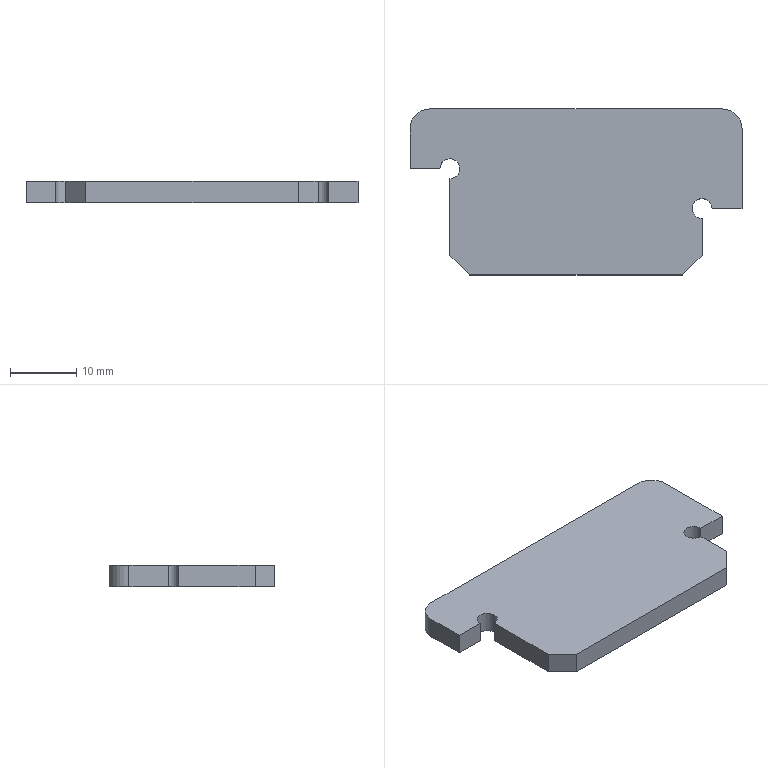Part | SolidWorks | features FlatPattern 1, SMBaseFlange 1, SheetMetal 1 | 1 solid | 17 faces | box 50 x 25 x 3.2 mm | volume 3426 mm3 | plane 12 | cylinder 5 | commonest cylinder face diameters 3 x3 6 x2
STEP:
#1=CARTESIAN_POINT('',(-86.411,-492.5,3.2));
#2=VERTEX_POINT('',#1);
#3=CARTESIAN_POINT('',(-83.411,-492.5,3.2));
#4=VERTEX_POINT('',#3);
#5=CARTESIAN_POINT('',(-84.911,-492.5,3.2));
#6=DIRECTION('',(0.,0.,-1.));
#7=DIRECTION('',(1.,0.,0.));
#8=AXIS2_PLACEMENT_3D('',#5,#6,#7);
#9=CIRCLE('',#8,1.5);
#10=EDGE_CURVE('',#2,#4,#9,.T.);
#11=ORIENTED_EDGE('',*,*,#10,.F.);
#12=CARTESIAN_POINT('',(-86.411,-492.5,0.));
#13=VERTEX_POINT('',#12);
#14=CARTESIAN_POINT('',(-86.411,-492.5,3.2));
#15=DIRECTION('',(0.,0.,-1.));
#16=VECTOR('',#15,1000.);
#17=LINE('',#14,#16);
#18=EDGE_CURVE('',#2,#13,#17,.T.);
#19=ORIENTED_EDGE('',*,*,#18,.T.);
#20=CARTESIAN_POINT('',(-83.411,-492.5,0.));
#21=VERTEX_POINT('',#20);
#22=CARTESIAN_POINT('',(-84.911,-492.5,0.));
#23=DIRECTION('',(0.,0.,-1.));
#24=DIRECTION('',(1.,0.,0.));
#25=AXIS2_PLACEMENT_3D('',#22,#23,#24);
#26=CIRCLE('',#25,1.5);
#27=EDGE_CURVE('',#13,#21,#26,.T.);
#28=ORIENTED_EDGE('',*,*,#27,.T.);
#29=CARTESIAN_POINT('',(-83.411,-492.5,3.2));
#30=DIRECTION('',(0.,0.,-1.));
#31=VECTOR('',#30,1000.);
#32=LINE('',#29,#31);
#33=EDGE_CURVE('',#4,#21,#32,.T.);
#34=ORIENTED_EDGE('',*,*,#33,.F.);
#35=EDGE_LOOP('',(#11,#19,#28,#34));
#36=FACE_OUTER_BOUND('',#35,.T.);
#37=CARTESIAN_POINT('',(-84.911,-492.5,3.2));
#38=DIRECTION('',(0.,0.,-1.));
#39=DIRECTION('',(-1.,0.,0.));
#40=AXIS2_PLACEMENT_3D('',#37,#38,#39);
#41=CYLINDRICAL_SURFACE('',#40,1.5);
#42=ADVANCED_FACE('',(#36),#41,.F.);
#43=CARTESIAN_POINT('',(-128.911,-486.5,0.));
#44=VERTEX_POINT('',#43);
#45=CARTESIAN_POINT('',(-124.411,-486.5,0.));
#46=VERTEX_POINT('',#45);
#47=CARTESIAN_POINT('',(-124.411,-486.5,0.));
#48=DIRECTION('',(1.,0.,0.));
#49=VECTOR('',#48,1000.);
#50=LINE('',#47,#49);
#51=EDGE_CURVE('',#44,#46,#50,.T.);
#52=ORIENTED_EDGE('',*,*,#51,.T.);
#53=CARTESIAN_POINT('',(-124.411,-486.5,3.2));
#54=VERTEX_POINT('',#53);
#55=CARTESIAN_POINT('',(-124.411,-486.5,3.2));
#56=DIRECTION('',(0.,0.,-1.));
#57=VECTOR('',#56,1000.);
#58=LINE('',#55,#57);
#59=EDGE_CURVE('',#54,#46,#58,.T.);
#60=ORIENTED_EDGE('',*,*,#59,.F.);
#61=CARTESIAN_POINT('',(-128.911,-486.5,3.2));
#62=VERTEX_POINT('',#61);
#63=CARTESIAN_POINT('',(-124.411,-486.5,3.2));
#64=DIRECTION('',(1.,0.,0.));
#65=VECTOR('',#64,1000.);
#66=LINE('',#63,#65);
#67=EDGE_CURVE('',#62,#54,#66,.T.);
#68=ORIENTED_EDGE('',*,*,#67,.F.);
#69=CARTESIAN_POINT('',(-128.911,-486.5,3.2));
#70=DIRECTION('',(0.,0.,-1.));
#71=VECTOR('',#70,1000.);
#72=LINE('',#69,#71);
#73=EDGE_CURVE('',#62,#44,#72,.T.);
#74=ORIENTED_EDGE('',*,*,#73,.T.);
#75=EDGE_LOOP('',(#52,#60,#68,#74));
#76=FACE_OUTER_BOUND('',#75,.T.);
#77=CARTESIAN_POINT('',(-124.411,-486.5,3.2));
#78=DIRECTION('',(0.,1.,0.));
#79=DIRECTION('',(0.,0.,1.));
#80=AXIS2_PLACEMENT_3D('',#77,#78,#79);
#81=PLANE('',#80);
#82=ADVANCED_FACE('',(#76),#81,.F.);
#83=CARTESIAN_POINT('',(-122.911,-488.,0.));
#84=VERTEX_POINT('',#83);
#85=CARTESIAN_POINT('',(-122.911,-486.5,0.));
#86=DIRECTION('',(0.,0.,-1.));
#87=DIRECTION('',(1.,0.,0.));
#88=AXIS2_PLACEMENT_3D('',#85,#86,#87);
#89=CIRCLE('',#88,1.5);
#90=EDGE_CURVE('',#46,#84,#89,.T.);
#91=ORIENTED_EDGE('',*,*,#90,.T.);
#92=CARTESIAN_POINT('',(-122.911,-488.,3.2));
#93=VERTEX_POINT('',#92);
#94=CARTESIAN_POINT('',(-122.911,-488.,3.2));
#95=DIRECTION('',(0.,0.,-1.));
#96=VECTOR('',#95,1000.);
#97=LINE('',#94,#96);
#98=EDGE_CURVE('',#93,#84,#97,.T.);
#99=ORIENTED_EDGE('',*,*,#98,.F.);
#100=CARTESIAN_POINT('',(-122.911,-486.5,3.2));
#101=DIRECTION('',(0.,0.,-1.));
#102=DIRECTION('',(1.,0.,0.));
#103=AXIS2_PLACEMENT_3D('',#100,#101,#102);
#104=CIRCLE('',#103,1.5);
#105=EDGE_CURVE('',#54,#93,#104,.T.);
#106=ORIENTED_EDGE('',*,*,#105,.F.);
#107=ORIENTED_EDGE('',*,*,#59,.T.);
#108=EDGE_LOOP('',(#91,#99,#106,#107));
#109=FACE_OUTER_BOUND('',#108,.T.);
#110=CARTESIAN_POINT('',(-122.911,-486.5,3.2));
#111=DIRECTION('',(0.,0.,-1.));
#112=DIRECTION('',(-1.,0.,0.));
#113=AXIS2_PLACEMENT_3D('',#110,#111,#112);
#114=CYLINDRICAL_SURFACE('',#113,1.5);
#115=ADVANCED_FACE('',(#109),#114,.F.);
#116=CARTESIAN_POINT('',(-122.911,-499.5,0.));
#117=VERTEX_POINT('',#116);
#118=CARTESIAN_POINT('',(-122.911,-499.5,0.));
#119=DIRECTION('',(0.,-1.,0.));
#120=VECTOR('',#119,1000.);
#121=LINE('',#118,#120);
#122=EDGE_CURVE('',#84,#117,#121,.T.);
#123=ORIENTED_EDGE('',*,*,#122,.T.);
#124=CARTESIAN_POINT('',(-122.911,-499.5,3.2));
#125=VERTEX_POINT('',#124);
#126=CARTESIAN_POINT('',(-122.911,-499.5,3.2));
#127=DIRECTION('',(0.,0.,-1.));
#128=VECTOR('',#127,1000.);
#129=LINE('',#126,#128);
#130=EDGE_CURVE('',#125,#117,#129,.T.);
#131=ORIENTED_EDGE('',*,*,#130,.F.);
#132=CARTESIAN_POINT('',(-122.911,-499.5,3.2));
#133=DIRECTION('',(0.,-1.,0.));
#134=VECTOR('',#133,1000.);
#135=LINE('',#132,#134);
#136=EDGE_CURVE('',#93,#125,#135,.T.);
#137=ORIENTED_EDGE('',*,*,#136,.F.);
#138=ORIENTED_EDGE('',*,*,#98,.T.);
#139=EDGE_LOOP('',(#123,#131,#137,#138));
#140=FACE_OUTER_BOUND('',#139,.T.);
#141=CARTESIAN_POINT('',(-122.911,-499.5,3.2));
#142=DIRECTION('',(1.,0.,0.));
#143=DIRECTION('',(0.,1.,0.));
#144=AXIS2_PLACEMENT_3D('',#141,#142,#143);
#145=PLANE('',#144);
#146=ADVANCED_FACE('',(#140),#145,.F.);
#147=CARTESIAN_POINT('',(-119.911,-502.5,0.));
#148=VERTEX_POINT('',#147);
#149=CARTESIAN_POINT('',(-119.911,-502.5,0.));
#150=DIRECTION('',(0.7071,-0.7071,0.));
#151=VECTOR('',#150,1000.);
#152=LINE('',#149,#151);
#153=EDGE_CURVE('',#117,#148,#152,.T.);
#154=ORIENTED_EDGE('',*,*,#153,.T.);
#155=CARTESIAN_POINT('',(-119.911,-502.5,3.2));
#156=VERTEX_POINT('',#155);
#157=CARTESIAN_POINT('',(-119.911,-502.5,3.2));
#158=DIRECTION('',(0.,0.,-1.));
#159=VECTOR('',#158,1000.);
#160=LINE('',#157,#159);
#161=EDGE_CURVE('',#156,#148,#160,.T.);
#162=ORIENTED_EDGE('',*,*,#161,.F.);
#163=CARTESIAN_POINT('',(-119.911,-502.5,3.2));
#164=DIRECTION('',(0.7071,-0.7071,0.));
#165=VECTOR('',#164,1000.);
#166=LINE('',#163,#165);
#167=EDGE_CURVE('',#125,#156,#166,.T.);
#168=ORIENTED_EDGE('',*,*,#167,.F.);
#169=ORIENTED_EDGE('',*,*,#130,.T.);
#170=EDGE_LOOP('',(#154,#162,#168,#169));
#171=FACE_OUTER_BOUND('',#170,.T.);
#172=CARTESIAN_POINT('',(-119.911,-502.5,3.2));
#173=DIRECTION('',(0.7071,0.7071,0.));
#174=DIRECTION('',(-0.7071,0.7071,0.));
#175=AXIS2_PLACEMENT_3D('',#172,#173,#174);
#176=PLANE('',#175);
#177=ADVANCED_FACE('',(#171),#176,.F.);
#178=CARTESIAN_POINT('',(-87.911,-502.5,0.));
#179=VERTEX_POINT('',#178);
#180=CARTESIAN_POINT('',(-87.911,-502.5,0.));
#181=DIRECTION('',(1.,0.,0.));
#182=VECTOR('',#181,1000.);
#183=LINE('',#180,#182);
#184=EDGE_CURVE('',#148,#179,#183,.T.);
#185=ORIENTED_EDGE('',*,*,#184,.T.);
#186=CARTESIAN_POINT('',(-87.911,-502.5,3.2));
#187=VERTEX_POINT('',#186);
#188=CARTESIAN_POINT('',(-87.911,-502.5,3.2));
#189=DIRECTION('',(0.,0.,-1.));
#190=VECTOR('',#189,1000.);
#191=LINE('',#188,#190);
#192=EDGE_CURVE('',#187,#179,#191,.T.);
#193=ORIENTED_EDGE('',*,*,#192,.F.);
#194=CARTESIAN_POINT('',(-87.911,-502.5,3.2));
#195=DIRECTION('',(1.,0.,0.));
#196=VECTOR('',#195,1000.);
#197=LINE('',#194,#196);
#198=EDGE_CURVE('',#156,#187,#197,.T.);
#199=ORIENTED_EDGE('',*,*,#198,.F.);
#200=ORIENTED_EDGE('',*,*,#161,.T.);
#201=EDGE_LOOP('',(#185,#193,#199,#200));
#202=FACE_OUTER_BOUND('',#201,.T.);
#203=CARTESIAN_POINT('',(-87.911,-502.5,3.2));
#204=DIRECTION('',(0.,1.,0.));
#205=DIRECTION('',(0.,0.,1.));
#206=AXIS2_PLACEMENT_3D('',#203,#204,#205);
#207=PLANE('',#206);
#208=ADVANCED_FACE('',(#202),#207,.F.);
#209=CARTESIAN_POINT('',(-84.911,-499.5,0.));
#210=VERTEX_POINT('',#209);
#211=CARTESIAN_POINT('',(-84.911,-499.5,0.));
#212=DIRECTION('',(0.7071,0.7071,0.));
#213=VECTOR('',#212,1000.);
#214=LINE('',#211,#213);
#215=EDGE_CURVE('',#179,#210,#214,.T.);
#216=ORIENTED_EDGE('',*,*,#215,.T.);
#217=CARTESIAN_POINT('',(-84.911,-499.5,3.2));
#218=VERTEX_POINT('',#217);
#219=CARTESIAN_POINT('',(-84.911,-499.5,3.2));
#220=DIRECTION('',(0.,0.,-1.));
#221=VECTOR('',#220,1000.);
#222=LINE('',#219,#221);
#223=EDGE_CURVE('',#218,#210,#222,.T.);
#224=ORIENTED_EDGE('',*,*,#223,.F.);
#225=CARTESIAN_POINT('',(-84.911,-499.5,3.2));
#226=DIRECTION('',(0.7071,0.7071,0.));
#227=VECTOR('',#226,1000.);
#228=LINE('',#225,#227);
#229=EDGE_CURVE('',#187,#218,#228,.T.);
#230=ORIENTED_EDGE('',*,*,#229,.F.);
#231=ORIENTED_EDGE('',*,*,#192,.T.);
#232=EDGE_LOOP('',(#216,#224,#230,#231));
#233=FACE_OUTER_BOUND('',#232,.T.);
#234=CARTESIAN_POINT('',(-84.911,-499.5,3.2));
#235=DIRECTION('',(-0.7071,0.7071,0.));
#236=DIRECTION('',(-0.7071,-0.7071,0.));
#237=AXIS2_PLACEMENT_3D('',#234,#235,#236);
#238=PLANE('',#237);
#239=ADVANCED_FACE('',(#233),#238,.F.);
#240=CARTESIAN_POINT('',(-84.911,-494.,0.));
#241=VERTEX_POINT('',#240);
#242=CARTESIAN_POINT('',(-84.911,-494.,0.));
#243=DIRECTION('',(0.,1.,0.));
#244=VECTOR('',#243,1000.);
#245=LINE('',#242,#244);
#246=EDGE_CURVE('',#210,#241,#245,.T.);
#247=ORIENTED_EDGE('',*,*,#246,.T.);
#248=CARTESIAN_POINT('',(-84.911,-494.,3.2));
#249=VERTEX_POINT('',#248);
#250=CARTESIAN_POINT('',(-84.911,-494.,3.2));
#251=DIRECTION('',(0.,0.,-1.));
#252=VECTOR('',#251,1000.);
#253=LINE('',#250,#252);
#254=EDGE_CURVE('',#249,#241,#253,.T.);
#255=ORIENTED_EDGE('',*,*,#254,.F.);
#256=CARTESIAN_POINT('',(-84.911,-494.,3.2));
#257=DIRECTION('',(0.,1.,0.));
#258=VECTOR('',#257,1000.);
#259=LINE('',#256,#258);
#260=EDGE_CURVE('',#218,#249,#259,.T.);
#261=ORIENTED_EDGE('',*,*,#260,.F.);
#262=ORIENTED_EDGE('',*,*,#223,.T.);
#263=EDGE_LOOP('',(#247,#255,#261,#262));
#264=FACE_OUTER_BOUND('',#263,.T.);
#265=CARTESIAN_POINT('',(-84.911,-494.,3.2));
#266=DIRECTION('',(-1.,0.,0.));
#267=DIRECTION('',(0.,0.,1.));
#268=AXIS2_PLACEMENT_3D('',#265,#266,#267);
#269=PLANE('',#268);
#270=ADVANCED_FACE('',(#264),#269,.F.);
#271=ORIENTED_EDGE('',*,*,#18,.F.);
#272=CARTESIAN_POINT('',(-84.911,-492.5,3.2));
#273=DIRECTION('',(0.,0.,-1.));
#274=DIRECTION('',(1.,0.,0.));
#275=AXIS2_PLACEMENT_3D('',#272,#273,#274);
#276=CIRCLE('',#275,1.5);
#277=EDGE_CURVE('',#249,#2,#276,.T.);
#278=ORIENTED_EDGE('',*,*,#277,.F.);
#279=ORIENTED_EDGE('',*,*,#254,.T.);
#280=CARTESIAN_POINT('',(-84.911,-492.5,0.));
#281=DIRECTION('',(0.,0.,-1.));
#282=DIRECTION('',(1.,0.,0.));
#283=AXIS2_PLACEMENT_3D('',#280,#281,#282);
#284=CIRCLE('',#283,1.5);
#285=EDGE_CURVE('',#241,#13,#284,.T.);
#286=ORIENTED_EDGE('',*,*,#285,.T.);
#287=EDGE_LOOP('',(#271,#278,#279,#286));
#288=FACE_OUTER_BOUND('',#287,.T.);
#289=CARTESIAN_POINT('',(-84.911,-492.5,3.2));
#290=DIRECTION('',(0.,0.,-1.));
#291=DIRECTION('',(-1.,0.,0.));
#292=AXIS2_PLACEMENT_3D('',#289,#290,#291);
#293=CYLINDRICAL_SURFACE('',#292,1.5);
#294=ADVANCED_FACE('',(#288),#293,.F.);
#295=CARTESIAN_POINT('',(-78.911,-492.5,0.));
#296=VERTEX_POINT('',#295);
#297=CARTESIAN_POINT('',(-78.911,-492.5,0.));
#298=DIRECTION('',(1.,0.,0.));
#299=VECTOR('',#298,1000.);
#300=LINE('',#297,#299);
#301=EDGE_CURVE('',#21,#296,#300,.T.);
#302=ORIENTED_EDGE('',*,*,#301,.T.);
#303=CARTESIAN_POINT('',(-78.911,-492.5,3.2));
#304=VERTEX_POINT('',#303);
#305=CARTESIAN_POINT('',(-78.911,-492.5,3.2));
#306=DIRECTION('',(0.,0.,-1.));
#307=VECTOR('',#306,1000.);
#308=LINE('',#305,#307);
#309=EDGE_CURVE('',#304,#296,#308,.T.);
#310=ORIENTED_EDGE('',*,*,#309,.F.);
#311=CARTESIAN_POINT('',(-78.911,-492.5,3.2));
#312=DIRECTION('',(1.,0.,0.));
#313=VECTOR('',#312,1000.);
#314=LINE('',#311,#313);
#315=EDGE_CURVE('',#4,#304,#314,.T.);
#316=ORIENTED_EDGE('',*,*,#315,.F.);
#317=ORIENTED_EDGE('',*,*,#33,.T.);
#318=EDGE_LOOP('',(#302,#310,#316,#317));
#319=FACE_OUTER_BOUND('',#318,.T.);
#320=CARTESIAN_POINT('',(-78.911,-492.5,3.2));
#321=DIRECTION('',(0.,1.,0.));
#322=DIRECTION('',(0.,0.,1.));
#323=AXIS2_PLACEMENT_3D('',#320,#321,#322);
#324=PLANE('',#323);
#325=ADVANCED_FACE('',(#319),#324,.F.);
#326=CARTESIAN_POINT('',(-78.911,-480.5,0.));
#327=VERTEX_POINT('',#326);
#328=CARTESIAN_POINT('',(-78.911,-480.5,0.));
#329=DIRECTION('',(0.,1.,0.));
#330=VECTOR('',#329,1000.);
#331=LINE('',#328,#330);
#332=EDGE_CURVE('',#296,#327,#331,.T.);
#333=ORIENTED_EDGE('',*,*,#332,.T.);
#334=CARTESIAN_POINT('',(-78.911,-480.5,3.2));
#335=VERTEX_POINT('',#334);
#336=CARTESIAN_POINT('',(-78.911,-480.5,3.2));
#337=DIRECTION('',(0.,0.,-1.));
#338=VECTOR('',#337,1000.);
#339=LINE('',#336,#338);
#340=EDGE_CURVE('',#335,#327,#339,.T.);
#341=ORIENTED_EDGE('',*,*,#340,.F.);
#342=CARTESIAN_POINT('',(-78.911,-480.5,3.2));
#343=DIRECTION('',(0.,1.,0.));
#344=VECTOR('',#343,1000.);
#345=LINE('',#342,#344);
#346=EDGE_CURVE('',#304,#335,#345,.T.);
#347=ORIENTED_EDGE('',*,*,#346,.F.);
#348=ORIENTED_EDGE('',*,*,#309,.T.);
#349=EDGE_LOOP('',(#333,#341,#347,#348));
#350=FACE_OUTER_BOUND('',#349,.T.);
#351=CARTESIAN_POINT('',(-78.911,-480.5,3.2));
#352=DIRECTION('',(-1.,0.,0.));
#353=DIRECTION('',(0.,0.,1.));
#354=AXIS2_PLACEMENT_3D('',#351,#352,#353);
#355=PLANE('',#354);
#356=ADVANCED_FACE('',(#350),#355,.F.);
#357=CARTESIAN_POINT('',(-81.911,-477.5,0.));
#358=VERTEX_POINT('',#357);
#359=CARTESIAN_POINT('',(-81.911,-480.5,0.));
#360=DIRECTION('',(0.,0.,1.));
#361=DIRECTION('',(-1.,0.,0.));
#362=AXIS2_PLACEMENT_3D('',#359,#360,#361);
#363=CIRCLE('',#362,3.);
#364=EDGE_CURVE('',#327,#358,#363,.T.);
#365=ORIENTED_EDGE('',*,*,#364,.T.);
#366=CARTESIAN_POINT('',(-81.911,-477.5,3.2));
#367=VERTEX_POINT('',#366);
#368=CARTESIAN_POINT('',(-81.911,-477.5,3.2));
#369=DIRECTION('',(0.,0.,-1.));
#370=VECTOR('',#369,1000.);
#371=LINE('',#368,#370);
#372=EDGE_CURVE('',#367,#358,#371,.T.);
#373=ORIENTED_EDGE('',*,*,#372,.F.);
#374=CARTESIAN_POINT('',(-81.911,-480.5,3.2));
#375=DIRECTION('',(0.,0.,1.));
#376=DIRECTION('',(-1.,0.,0.));
#377=AXIS2_PLACEMENT_3D('',#374,#375,#376);
#378=CIRCLE('',#377,3.);
#379=EDGE_CURVE('',#335,#367,#378,.T.);
#380=ORIENTED_EDGE('',*,*,#379,.F.);
#381=ORIENTED_EDGE('',*,*,#340,.T.);
#382=EDGE_LOOP('',(#365,#373,#380,#381));
#383=FACE_OUTER_BOUND('',#382,.T.);
#384=CARTESIAN_POINT('',(-81.911,-480.5,3.2));
#385=DIRECTION('',(0.,0.,-1.));
#386=DIRECTION('',(-1.,0.,0.));
#387=AXIS2_PLACEMENT_3D('',#384,#385,#386);
#388=CYLINDRICAL_SURFACE('',#387,3.);
#389=ADVANCED_FACE('',(#383),#388,.T.);
#390=CARTESIAN_POINT('',(-125.911,-477.5,0.));
#391=VERTEX_POINT('',#390);
#392=CARTESIAN_POINT('',(-125.911,-477.5,0.));
#393=DIRECTION('',(-1.,0.,0.));
#394=VECTOR('',#393,1000.);
#395=LINE('',#392,#394);
#396=EDGE_CURVE('',#358,#391,#395,.T.);
#397=ORIENTED_EDGE('',*,*,#396,.T.);
#398=CARTESIAN_POINT('',(-125.911,-477.5,3.2));
#399=VERTEX_POINT('',#398);
#400=CARTESIAN_POINT('',(-125.911,-477.5,3.2));
#401=DIRECTION('',(0.,0.,-1.));
#402=VECTOR('',#401,1000.);
#403=LINE('',#400,#402);
#404=EDGE_CURVE('',#399,#391,#403,.T.);
#405=ORIENTED_EDGE('',*,*,#404,.F.);
#406=CARTESIAN_POINT('',(-125.911,-477.5,3.2));
#407=DIRECTION('',(-1.,0.,0.));
#408=VECTOR('',#407,1000.);
#409=LINE('',#406,#408);
#410=EDGE_CURVE('',#367,#399,#409,.T.);
#411=ORIENTED_EDGE('',*,*,#410,.F.);
#412=ORIENTED_EDGE('',*,*,#372,.T.);
#413=EDGE_LOOP('',(#397,#405,#411,#412));
#414=FACE_OUTER_BOUND('',#413,.T.);
#415=CARTESIAN_POINT('',(-125.911,-477.5,3.2));
#416=DIRECTION('',(0.,-1.,0.));
#417=DIRECTION('',(0.,0.,-1.));
#418=AXIS2_PLACEMENT_3D('',#415,#416,#417);
#419=PLANE('',#418);
#420=ADVANCED_FACE('',(#414),#419,.F.);
#421=CARTESIAN_POINT('',(-128.911,-480.5,0.));
#422=VERTEX_POINT('',#421);
#423=CARTESIAN_POINT('',(-125.911,-480.5,0.));
#424=DIRECTION('',(0.,0.,1.));
#425=DIRECTION('',(-1.,0.,0.));
#426=AXIS2_PLACEMENT_3D('',#423,#424,#425);
#427=CIRCLE('',#426,3.);
#428=EDGE_CURVE('',#391,#422,#427,.T.);
#429=ORIENTED_EDGE('',*,*,#428,.T.);
#430=CARTESIAN_POINT('',(-128.911,-480.5,3.2));
#431=VERTEX_POINT('',#430);
#432=CARTESIAN_POINT('',(-128.911,-480.5,3.2));
#433=DIRECTION('',(0.,0.,-1.));
#434=VECTOR('',#433,1000.);
#435=LINE('',#432,#434);
#436=EDGE_CURVE('',#431,#422,#435,.T.);
#437=ORIENTED_EDGE('',*,*,#436,.F.);
#438=CARTESIAN_POINT('',(-125.911,-480.5,3.2));
#439=DIRECTION('',(0.,0.,1.));
#440=DIRECTION('',(-1.,0.,0.));
#441=AXIS2_PLACEMENT_3D('',#438,#439,#440);
#442=CIRCLE('',#441,3.);
#443=EDGE_CURVE('',#399,#431,#442,.T.);
#444=ORIENTED_EDGE('',*,*,#443,.F.);
#445=ORIENTED_EDGE('',*,*,#404,.T.);
#446=EDGE_LOOP('',(#429,#437,#444,#445));
#447=FACE_OUTER_BOUND('',#446,.T.);
#448=CARTESIAN_POINT('',(-125.911,-480.5,3.2));
#449=DIRECTION('',(0.,0.,-1.));
#450=DIRECTION('',(-1.,0.,0.));
#451=AXIS2_PLACEMENT_3D('',#448,#449,#450);
#452=CYLINDRICAL_SURFACE('',#451,3.);
#453=ADVANCED_FACE('',(#447),#452,.T.);
#454=CARTESIAN_POINT('',(-128.911,-486.5,0.));
#455=DIRECTION('',(0.,-1.,0.));
#456=VECTOR('',#455,1000.);
#457=LINE('',#454,#456);
#458=EDGE_CURVE('',#422,#44,#457,.T.);
#459=ORIENTED_EDGE('',*,*,#458,.T.);
#460=ORIENTED_EDGE('',*,*,#73,.F.);
#461=CARTESIAN_POINT('',(-128.911,-486.5,3.2));
#462=DIRECTION('',(0.,-1.,0.));
#463=VECTOR('',#462,1000.);
#464=LINE('',#461,#463);
#465=EDGE_CURVE('',#431,#62,#464,.T.);
#466=ORIENTED_EDGE('',*,*,#465,.F.);
#467=ORIENTED_EDGE('',*,*,#436,.T.);
#468=EDGE_LOOP('',(#459,#460,#466,#467));
#469=FACE_OUTER_BOUND('',#468,.T.);
#470=CARTESIAN_POINT('',(-128.911,-486.5,3.2));
#471=DIRECTION('',(1.,0.,0.));
#472=DIRECTION('',(0.,0.,-1.));
#473=AXIS2_PLACEMENT_3D('',#470,#471,#472);
#474=PLANE('',#473);
#475=ADVANCED_FACE('',(#469),#474,.F.);
#476=ORIENTED_EDGE('',*,*,#67,.T.);
#477=ORIENTED_EDGE('',*,*,#105,.T.);
#478=ORIENTED_EDGE('',*,*,#136,.T.);
#479=ORIENTED_EDGE('',*,*,#167,.T.);
#480=ORIENTED_EDGE('',*,*,#198,.T.);
#481=ORIENTED_EDGE('',*,*,#229,.T.);
#482=ORIENTED_EDGE('',*,*,#260,.T.);
#483=ORIENTED_EDGE('',*,*,#277,.T.);
#484=ORIENTED_EDGE('',*,*,#10,.T.);
#485=ORIENTED_EDGE('',*,*,#315,.T.);
#486=ORIENTED_EDGE('',*,*,#346,.T.);
#487=ORIENTED_EDGE('',*,*,#379,.T.);
#488=ORIENTED_EDGE('',*,*,#410,.T.);
#489=ORIENTED_EDGE('',*,*,#443,.T.);
#490=ORIENTED_EDGE('',*,*,#465,.T.);
#491=EDGE_LOOP('',(#476,#477,#478,#479,#480,#481,#482,#483,#484,#485,#486,#487,#488,#489,#490));
#492=FACE_OUTER_BOUND('',#491,.T.);
#493=CARTESIAN_POINT('',(-125.911,-480.5,3.2));
#494=DIRECTION('',(0.,0.,-1.));
#495=DIRECTION('',(-1.,0.,0.));
#496=AXIS2_PLACEMENT_3D('',#493,#494,#495);
#497=PLANE('',#496);
#498=ADVANCED_FACE('',(#492),#497,.F.);
#499=ORIENTED_EDGE('',*,*,#51,.F.);
#500=ORIENTED_EDGE('',*,*,#458,.F.);
#501=ORIENTED_EDGE('',*,*,#428,.F.);
#502=ORIENTED_EDGE('',*,*,#396,.F.);
#503=ORIENTED_EDGE('',*,*,#364,.F.);
#504=ORIENTED_EDGE('',*,*,#332,.F.);
#505=ORIENTED_EDGE('',*,*,#301,.F.);
#506=ORIENTED_EDGE('',*,*,#27,.F.);
#507=ORIENTED_EDGE('',*,*,#285,.F.);
#508=ORIENTED_EDGE('',*,*,#246,.F.);
#509=ORIENTED_EDGE('',*,*,#215,.F.);
#510=ORIENTED_EDGE('',*,*,#184,.F.);
#511=ORIENTED_EDGE('',*,*,#153,.F.);
#512=ORIENTED_EDGE('',*,*,#122,.F.);
#513=ORIENTED_EDGE('',*,*,#90,.F.);
#514=EDGE_LOOP('',(#499,#500,#501,#502,#503,#504,#505,#506,#507,#508,#509,#510,#511,#512,#513));
#515=FACE_OUTER_BOUND('',#514,.T.);
#516=CARTESIAN_POINT('',(-125.911,-480.5,0.));
#517=DIRECTION('',(0.,0.,-1.));
#518=DIRECTION('',(-1.,0.,0.));
#519=AXIS2_PLACEMENT_3D('',#516,#517,#518);
#520=PLANE('',#519);
#521=ADVANCED_FACE('',(#515),#520,.T.);
#522=CLOSED_SHELL('',(#42,#82,#115,#146,#177,#208,#239,#270,#294,#325,#356,#389,#420,#453,#475,#498,#521));
#523=MANIFOLD_SOLID_BREP('',#522);
#524=CARTESIAN_POINT('',(0.,0.,0.));
#525=DIRECTION('',(0.,0.,1.));
#526=DIRECTION('',(1.,0.,0.));
#527=AXIS2_PLACEMENT_3D('',#524,#525,#526);
#528=(LENGTH_UNIT()NAMED_UNIT(*)SI_UNIT(.MILLI.,.METRE.));
#529=UNCERTAINTY_MEASURE_WITH_UNIT(LENGTH_MEASURE(0.00001),#528,'','');
#530=(NAMED_UNIT(*)PLANE_ANGLE_UNIT()SI_UNIT($,.RADIAN.));
#531=(NAMED_UNIT(*)SI_UNIT($,.STERADIAN.)SOLID_ANGLE_UNIT());
#532=(GEOMETRIC_REPRESENTATION_CONTEXT(3)GLOBAL_UNCERTAINTY_ASSIGNED_CONTEXT((#529))GLOBAL_UNIT_ASSIGNED_CONTEXT((#528,#530,#531))REPRESENTATION_CONTEXT('',''));
#533=ADVANCED_BREP_SHAPE_REPRESENTATION('',(#523,#527),#532);